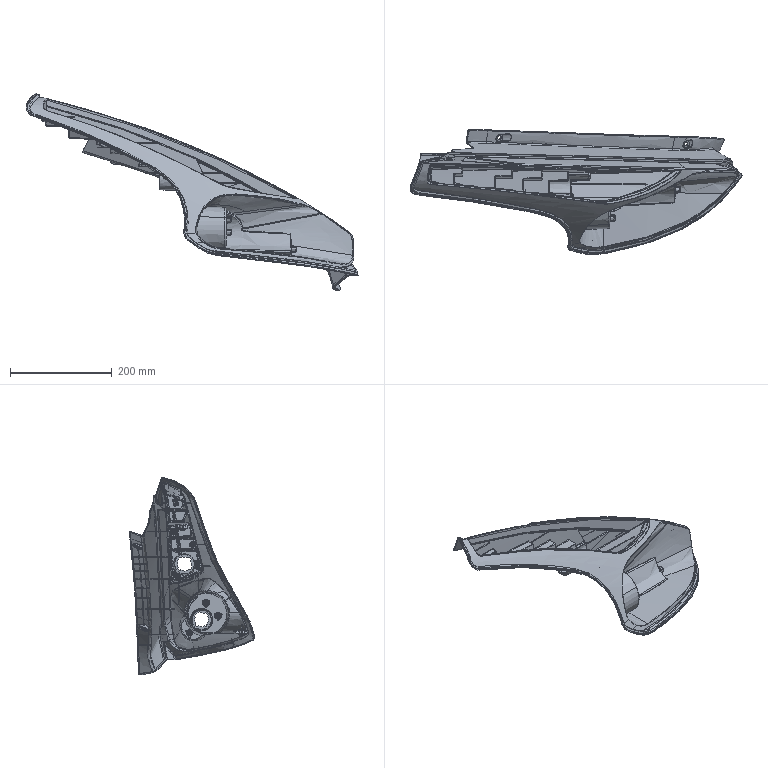Part | STEP file | solid 268 | 1 solid | 1864 faces | box 652.466 x 245.902 x 388.968 mm | volume 650950 mm3 | spline 1378 | plane 229 | sphere 85 | cylinder 78 | torus 44 | cone 43 | other 7 | commonest cylinder face diameters 4.02 x21 2.01 x17 27.135 x8 31.155 x8 2.915 x7 1.005 x6